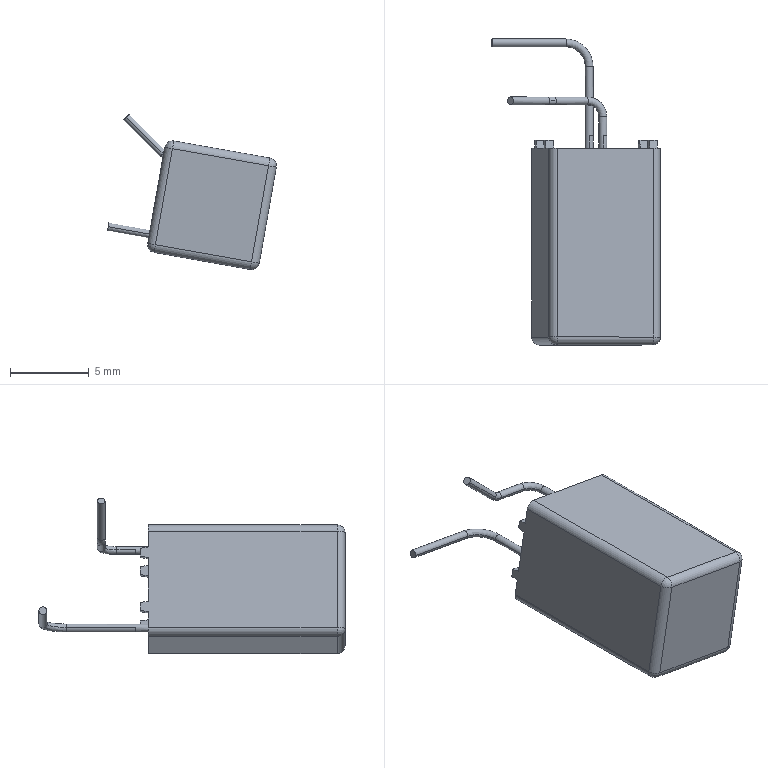Part | SolidWorks | features BaseBody 1 | 1 solid | 55 faces | box 10.728 x 19.45 x 9.871 mm | volume 648.732 mm3 | plane 24 | cylinder 20 | torus 7 | sphere 4 | commonest cylinder face diameters 0.5 x12 1 x8